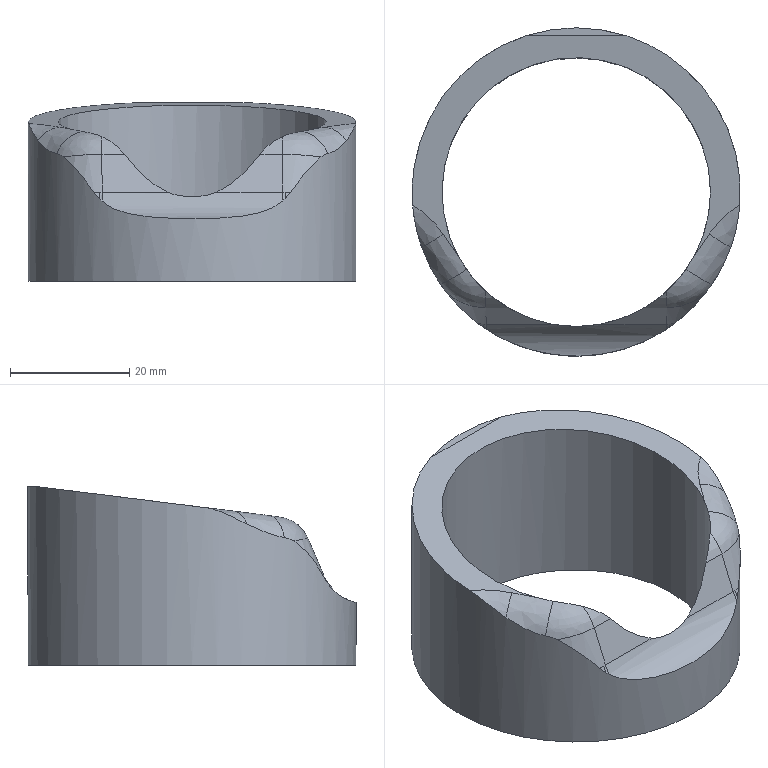Part | NX | features solid 2 | 1 solid | 22 faces | box 55 x 55 x 30 mm | volume 19165 mm3 | spline 10 | cylinder 7 | plane 5 | commonest cylinder face diameters 12 x2 20 x2 15 x1 45 x1 55 x1
STEP:
#1=CARTESIAN_POINT('',(-336.497,-154.34,29.));
#2=VERTEX_POINT('',#1);
#3=CARTESIAN_POINT('',(-353.503,-154.34,29.));
#4=VERTEX_POINT('',#3);
#5=CARTESIAN_POINT('',(-345.,-154.34,29.));
#6=DIRECTION('',(1.,0.,0.));
#7=VECTOR('',#6,1000.);
#8=LINE('',#5,#7);
#9=EDGE_CURVE('',#2,#4,#8,.F.);
#10=ORIENTED_EDGE('',*,*,#9,.F.);
#11=CARTESIAN_POINT('',(-345.,-180.493,29.));
#12=DIRECTION('',(0.,0.,1.));
#13=DIRECTION('',(1.,0.,0.));
#14=AXIS2_PLACEMENT_3D('',#11,#12,#13);
#15=CIRCLE('',#14,27.5);
#16=EDGE_CURVE('',#4,#2,#15,.F.);
#17=ORIENTED_EDGE('',*,*,#16,.F.);
#18=EDGE_LOOP('',(#10,#17));
#19=FACE_BOUND('',#18,.T.);
#20=CARTESIAN_POINT('',(-345.,-180.493,29.));
#21=DIRECTION('',(0.,0.,1.));
#22=DIRECTION('',(1.,0.,0.));
#23=AXIS2_PLACEMENT_3D('',#20,#21,#22);
#24=PLANE('',#23);
#25=ADVANCED_FACE('',(#19),#24,.T.);
#26=CARTESIAN_POINT('',(-322.5,-180.493,-1.));
#27=VERTEX_POINT('',#26);
#28=CARTESIAN_POINT('',(-345.,-180.493,-1.));
#29=DIRECTION('',(0.,0.,1.));
#30=DIRECTION('',(1.,0.,0.));
#31=AXIS2_PLACEMENT_3D('',#28,#29,#30);
#32=CIRCLE('',#31,22.5);
#33=EDGE_CURVE('',#27,#27,#32,.F.);
#34=ORIENTED_EDGE('',*,*,#33,.T.);
#35=EDGE_LOOP('',(#34));
#36=FACE_BOUND('',#35,.T.);
#37=CARTESIAN_POINT('',(-325.178,-191.138,24.41));
#38=VERTEX_POINT('',#37);
#39=CARTESIAN_POINT('',(-325.175,-191.134,24.41));
#40=VERTEX_POINT('',#39);
#41=CARTESIAN_POINT('',(-325.178,-191.138,24.41));
#42=CARTESIAN_POINT('',(-325.177,-191.137,24.41));
#43=CARTESIAN_POINT('',(-325.176,-191.135,24.41));
#44=CARTESIAN_POINT('',(-325.176,-191.134,24.41));
#45=B_SPLINE_CURVE_WITH_KNOTS('',3,(#41,#42,#43,#44),.UNSPECIFIED.,.F.,.F.,(4,4),(0.,1.),.UNSPECIFIED.);
#46=EDGE_CURVE('',#38,#40,#45,.T.);
#47=ORIENTED_EDGE('',*,*,#46,.T.);
#48=CARTESIAN_POINT('',(-364.825,-191.134,24.41));
#49=VERTEX_POINT('',#48);
#50=CARTESIAN_POINT('',(-345.,-180.493,25.738));
#51=DIRECTION('',(0.,-0.1238,0.9923));
#52=DIRECTION('',(0.,0.9923,0.1238));
#53=AXIS2_PLACEMENT_3D('',#50,#51,#52);
#54=ELLIPSE('',#53,22.674,22.5);
#55=EDGE_CURVE('',#40,#49,#54,.T.);
#56=ORIENTED_EDGE('',*,*,#55,.T.);
#57=CARTESIAN_POINT('',(-364.822,-191.138,24.41));
#58=VERTEX_POINT('',#57);
#59=CARTESIAN_POINT('',(-364.825,-191.134,24.41));
#60=CARTESIAN_POINT('',(-364.824,-191.135,24.41));
#61=CARTESIAN_POINT('',(-364.823,-191.136,24.41));
#62=CARTESIAN_POINT('',(-364.822,-191.138,24.41));
#63=B_SPLINE_CURVE_WITH_KNOTS('',3,(#59,#60,#61,#62),.UNSPECIFIED.,.F.,.F.,(4,4),(0.,1.),.UNSPECIFIED.);
#64=EDGE_CURVE('',#49,#58,#63,.T.);
#65=ORIENTED_EDGE('',*,*,#64,.T.);
#66=CARTESIAN_POINT('',(-363.388,-193.46,24.119));
#67=VERTEX_POINT('',#66);
#68=CARTESIAN_POINT('',(-364.822,-191.138,24.41));
#69=CARTESIAN_POINT('',(-364.391,-191.94,24.309));
#70=CARTESIAN_POINT('',(-363.913,-192.714,24.211));
#71=CARTESIAN_POINT('',(-363.388,-193.46,24.119));
#72=B_SPLINE_CURVE_WITH_KNOTS('',3,(#68,#69,#70,#71),.UNSPECIFIED.,.F.,.F.,(4,4),(0.000004606,0.00275),.UNSPECIFIED.);
#73=EDGE_CURVE('',#58,#67,#72,.T.);
#74=ORIENTED_EDGE('',*,*,#73,.T.);
#75=CARTESIAN_POINT('',(-360.131,-197.145,23.293));
#76=VERTEX_POINT('',#75);
#77=CARTESIAN_POINT('',(-363.388,-193.46,24.119));
#78=CARTESIAN_POINT('',(-362.429,-194.818,23.95));
#79=CARTESIAN_POINT('',(-361.302,-196.081,23.84));
#80=CARTESIAN_POINT('',(-360.131,-197.145,23.293));
#81=B_SPLINE_CURVE_WITH_KNOTS('',3,(#77,#78,#79,#80),.UNSPECIFIED.,.F.,.F.,(4,4),(0.,0.005011),.UNSPECIFIED.);
#82=EDGE_CURVE('',#67,#76,#81,.T.);
#83=ORIENTED_EDGE('',*,*,#82,.T.);
#84=CARTESIAN_POINT('',(-356.336,-199.928,20.3));
#85=VERTEX_POINT('',#84);
#86=CARTESIAN_POINT('',(-360.131,-197.145,23.293));
#87=CARTESIAN_POINT('',(-359.468,-197.747,22.984));
#88=CARTESIAN_POINT('',(-358.149,-198.805,22.193));
#89=CARTESIAN_POINT('',(-356.866,-199.619,21.027));
#90=CARTESIAN_POINT('',(-356.336,-199.928,20.3));
#91=B_SPLINE_CURVE_WITH_KNOTS('',3,(#86,#87,#88,#89,#90),.UNSPECIFIED.,.F.,.F.,(4,1,4),(0.,0.002803,0.005605),.UNSPECIFIED.);
#92=EDGE_CURVE('',#76,#85,#91,.T.);
#93=ORIENTED_EDGE('',*,*,#92,.T.);
#94=CARTESIAN_POINT('',(-349.112,-202.614,13.973));
#95=VERTEX_POINT('',#94);
#96=CARTESIAN_POINT('',(-345.,-180.493,66.089));
#97=DIRECTION('',(0.,0.9205,-0.3907));
#98=DIRECTION('',(0.,0.3907,0.9205));
#99=AXIS2_PLACEMENT_3D('',#96,#97,#98);
#100=ELLIPSE('',#99,57.586,22.5);
#101=EDGE_CURVE('',#95,#85,#100,.T.);
#102=ORIENTED_EDGE('',*,*,#101,.F.);
#103=CARTESIAN_POINT('',(-340.888,-202.614,13.973));
#104=VERTEX_POINT('',#103);
#105=CARTESIAN_POINT('',(-340.888,-202.614,13.973));
#106=CARTESIAN_POINT('',(-342.176,-202.853,13.409));
#107=CARTESIAN_POINT('',(-344.991,-203.132,13.001));
#108=CARTESIAN_POINT('',(-347.826,-202.853,13.41));
#109=CARTESIAN_POINT('',(-349.112,-202.614,13.973));
#110=B_SPLINE_CURVE_WITH_KNOTS('',3,(#105,#106,#107,#108,#109),.UNSPECIFIED.,.F.,.F.,(4,1,4),(0.,0.004206,0.008413),.UNSPECIFIED.);
#111=EDGE_CURVE('',#104,#95,#110,.T.);
#112=ORIENTED_EDGE('',*,*,#111,.F.);
#113=CARTESIAN_POINT('',(-333.664,-199.928,20.3));
#114=VERTEX_POINT('',#113);
#115=CARTESIAN_POINT('',(-345.,-180.493,66.089));
#116=DIRECTION('',(0.,0.9205,-0.3907));
#117=DIRECTION('',(0.,0.3907,0.9205));
#118=AXIS2_PLACEMENT_3D('',#115,#116,#117);
#119=ELLIPSE('',#118,57.586,22.5);
#120=EDGE_CURVE('',#114,#104,#119,.T.);
#121=ORIENTED_EDGE('',*,*,#120,.F.);
#122=CARTESIAN_POINT('',(-329.869,-197.145,23.293));
#123=VERTEX_POINT('',#122);
#124=CARTESIAN_POINT('',(-333.664,-199.928,20.3));
#125=CARTESIAN_POINT('',(-332.603,-199.309,21.757));
#126=CARTESIAN_POINT('',(-331.194,-198.348,22.676));
#127=CARTESIAN_POINT('',(-329.869,-197.145,23.293));
#128=B_SPLINE_CURVE_WITH_KNOTS('',3,(#124,#125,#126,#127),.UNSPECIFIED.,.F.,.F.,(4,4),(0.,0.00561),.UNSPECIFIED.);
#129=EDGE_CURVE('',#114,#123,#128,.T.);
#130=ORIENTED_EDGE('',*,*,#129,.T.);
#131=CARTESIAN_POINT('',(-326.612,-193.46,24.119));
#132=VERTEX_POINT('',#131);
#133=CARTESIAN_POINT('',(-329.869,-197.145,23.293));
#134=CARTESIAN_POINT('',(-328.699,-196.082,23.839));
#135=CARTESIAN_POINT('',(-327.57,-194.818,23.95));
#136=CARTESIAN_POINT('',(-326.612,-193.46,24.119));
#137=B_SPLINE_CURVE_WITH_KNOTS('',3,(#133,#134,#135,#136),.UNSPECIFIED.,.F.,.F.,(4,4),(0.,0.005002),.UNSPECIFIED.);
#138=EDGE_CURVE('',#123,#132,#137,.T.);
#139=ORIENTED_EDGE('',*,*,#138,.T.);
#140=CARTESIAN_POINT('',(-326.612,-193.46,24.119));
#141=CARTESIAN_POINT('',(-326.087,-192.715,24.211));
#142=CARTESIAN_POINT('',(-325.609,-191.941,24.309));
#143=CARTESIAN_POINT('',(-325.178,-191.138,24.41));
#144=B_SPLINE_CURVE_WITH_KNOTS('',3,(#140,#141,#142,#143),.UNSPECIFIED.,.F.,.F.,(4,4),(0.,0.002745),.UNSPECIFIED.);
#145=EDGE_CURVE('',#132,#38,#144,.T.);
#146=ORIENTED_EDGE('',*,*,#145,.T.);
#147=EDGE_LOOP('',(#47,#56,#65,#74,#83,#93,#102,#112,#121,#130,#139,#146));
#148=FACE_BOUND('',#147,.T.);
#149=CARTESIAN_POINT('',(-345.,-180.493,-1.));
#150=DIRECTION('',(0.,0.,1.));
#151=DIRECTION('',(1.,0.,0.));
#152=AXIS2_PLACEMENT_3D('',#149,#150,#151);
#153=CYLINDRICAL_SURFACE('',#152,22.5);
#154=ADVANCED_FACE('',(#36,#148),#153,.F.);
#155=CARTESIAN_POINT('',(-372.5,-180.493,-1.));
#156=VERTEX_POINT('',#155);
#157=CARTESIAN_POINT('',(-345.,-180.493,-1.));
#158=DIRECTION('',(0.,0.,-1.));
#159=DIRECTION('',(-1.,0.,0.));
#160=AXIS2_PLACEMENT_3D('',#157,#158,#159);
#161=CIRCLE('',#160,27.5);
#162=EDGE_CURVE('',#156,#156,#161,.T.);
#163=ORIENTED_EDGE('',*,*,#162,.F.);
#164=EDGE_LOOP('',(#163));
#165=FACE_BOUND('',#164,.T.);
#166=CARTESIAN_POINT('',(-372.414,-182.672,25.466));
#167=VERTEX_POINT('',#166);
#168=CARTESIAN_POINT('',(-345.,-180.493,25.738));
#169=DIRECTION('',(0.,-0.1238,0.9923));
#170=DIRECTION('',(0.,0.9923,0.1238));
#171=AXIS2_PLACEMENT_3D('',#168,#169,#170);
#172=ELLIPSE('',#171,27.713,27.5);
#173=EDGE_CURVE('',#4,#167,#172,.T.);
#174=ORIENTED_EDGE('',*,*,#173,.F.);
#175=ORIENTED_EDGE('',*,*,#16,.T.);
#176=CARTESIAN_POINT('',(-317.585,-182.649,25.469));
#177=VERTEX_POINT('',#176);
#178=CARTESIAN_POINT('',(-345.,-180.493,25.738));
#179=DIRECTION('',(0.,-0.1238,0.9923));
#180=DIRECTION('',(0.,0.9923,0.1238));
#181=AXIS2_PLACEMENT_3D('',#178,#179,#180);
#182=ELLIPSE('',#181,27.713,27.5);
#183=EDGE_CURVE('',#177,#2,#182,.T.);
#184=ORIENTED_EDGE('',*,*,#183,.F.);
#185=CARTESIAN_POINT('',(-319.108,-189.759,22.675));
#186=VERTEX_POINT('',#185);
#187=CARTESIAN_POINT('',(-319.108,-189.759,22.675));
#188=CARTESIAN_POINT('',(-318.29,-187.473,23.676));
#189=CARTESIAN_POINT('',(-317.79,-185.264,25.142));
#190=CARTESIAN_POINT('',(-317.585,-182.649,25.469));
#191=B_SPLINE_CURVE_WITH_KNOTS('',3,(#187,#188,#189,#190),.UNSPECIFIED.,.F.,.F.,(4,4),(0.,0.007856),.UNSPECIFIED.);
#192=EDGE_CURVE('',#186,#177,#191,.T.);
#193=ORIENTED_EDGE('',*,*,#192,.F.);
#194=CARTESIAN_POINT('',(-322.27,-195.971,20.446));
#195=VERTEX_POINT('',#194);
#196=CARTESIAN_POINT('',(-322.27,-195.971,20.446));
#197=CARTESIAN_POINT('',(-320.893,-193.95,20.709));
#198=CARTESIAN_POINT('',(-319.874,-191.897,21.738));
#199=CARTESIAN_POINT('',(-319.108,-189.759,22.675));
#200=B_SPLINE_CURVE_WITH_KNOTS('',3,(#196,#197,#198,#199),.UNSPECIFIED.,.F.,.F.,(4,4),(0.,0.007347),.UNSPECIFIED.);
#201=EDGE_CURVE('',#195,#186,#200,.T.);
#202=ORIENTED_EDGE('',*,*,#201,.F.);
#203=CARTESIAN_POINT('',(-323.445,-197.569,19.879));
#204=VERTEX_POINT('',#203);
#205=CARTESIAN_POINT('',(-323.446,-197.571,19.878));
#206=CARTESIAN_POINT('',(-323.058,-197.082,20.202));
#207=CARTESIAN_POINT('',(-322.661,-196.546,20.37));
#208=CARTESIAN_POINT('',(-322.27,-195.971,20.446));
#209=B_SPLINE_CURVE_WITH_KNOTS('',3,(#205,#206,#207,#208),.UNSPECIFIED.,.F.,.F.,(4,4),(0.,0.002064),.UNSPECIFIED.);
#210=EDGE_CURVE('',#204,#195,#209,.T.);
#211=ORIENTED_EDGE('',*,*,#210,.F.);
#212=CARTESIAN_POINT('',(-328.545,-202.527,13.948));
#213=VERTEX_POINT('',#212);
#214=CARTESIAN_POINT('',(-328.546,-202.527,13.947));
#215=CARTESIAN_POINT('',(-327.725,-201.914,15.109));
#216=CARTESIAN_POINT('',(-326.053,-200.526,17.284));
#217=CARTESIAN_POINT('',(-324.311,-198.663,19.156));
#218=CARTESIAN_POINT('',(-323.443,-197.568,19.88));
#219=B_SPLINE_CURVE_WITH_KNOTS('',3,(#214,#215,#216,#217,#218),.UNSPECIFIED.,.F.,.F.,(4,1,4),(0.002663,0.007292,0.01192),.UNSPECIFIED.);
#220=EDGE_CURVE('',#213,#204,#219,.T.);
#221=ORIENTED_EDGE('',*,*,#220,.F.);
#222=CARTESIAN_POINT('',(-329.415,-203.15,12.923));
#223=VERTEX_POINT('',#222);
#224=CARTESIAN_POINT('',(-328.545,-202.526,13.948));
#225=CARTESIAN_POINT('',(-328.808,-202.723,13.576));
#226=CARTESIAN_POINT('',(-329.103,-202.935,13.242));
#227=CARTESIAN_POINT('',(-329.415,-203.15,12.923));
#228=B_SPLINE_CURVE_WITH_KNOTS('',3,(#224,#225,#226,#227),.UNSPECIFIED.,.F.,.F.,(4,4),(0.,0.001482),.UNSPECIFIED.);
#229=EDGE_CURVE('',#213,#223,#228,.T.);
#230=ORIENTED_EDGE('',*,*,#229,.T.);
#231=CARTESIAN_POINT('',(-329.884,-203.466,12.473));
#232=VERTEX_POINT('',#231);
#233=CARTESIAN_POINT('',(-329.415,-203.15,12.923));
#234=CARTESIAN_POINT('',(-329.567,-203.254,12.768));
#235=CARTESIAN_POINT('',(-329.723,-203.36,12.618));
#236=CARTESIAN_POINT('',(-329.884,-203.466,12.473));
#237=B_SPLINE_CURVE_WITH_KNOTS('',3,(#233,#234,#235,#236),.UNSPECIFIED.,.F.,.F.,(4,4),(0.,0.0007229),.UNSPECIFIED.);
#238=EDGE_CURVE('',#223,#232,#237,.T.);
#239=ORIENTED_EDGE('',*,*,#238,.T.);
#240=CARTESIAN_POINT('',(-360.116,-203.466,12.473));
#241=VERTEX_POINT('',#240);
#242=CARTESIAN_POINT('',(-329.884,-203.466,12.473));
#243=CARTESIAN_POINT('',(-330.82,-204.081,11.633));
#244=CARTESIAN_POINT('',(-333.044,-205.367,10.549));
#245=CARTESIAN_POINT('',(-338.129,-207.366,9.625));
#246=CARTESIAN_POINT('',(-343.602,-208.202,9.529));
#247=CARTESIAN_POINT('',(-349.134,-207.783,9.598));
#248=CARTESIAN_POINT('',(-353.106,-206.876,9.848));
#249=CARTESIAN_POINT('',(-356.94,-205.377,10.543));
#250=CARTESIAN_POINT('',(-359.182,-204.08,11.634));
#251=CARTESIAN_POINT('',(-360.116,-203.466,12.473));
#252=B_SPLINE_CURVE_WITH_KNOTS('',3,(#242,#243,#244,#245,#246,#247,#248,#249,#250,#251),.UNSPECIFIED.,.F.,.F.,(4,1,1,1,1,1,1,4),(0.,0.00412,0.00824,0.01648,0.0206,0.02472,0.02884,0.03296),.UNSPECIFIED.);
#253=EDGE_CURVE('',#232,#241,#252,.T.);
#254=ORIENTED_EDGE('',*,*,#253,.T.);
#255=CARTESIAN_POINT('',(-360.585,-203.15,12.923));
#256=VERTEX_POINT('',#255);
#257=CARTESIAN_POINT('',(-360.116,-203.466,12.473));
#258=CARTESIAN_POINT('',(-360.277,-203.36,12.618));
#259=CARTESIAN_POINT('',(-360.433,-203.254,12.768));
#260=CARTESIAN_POINT('',(-360.585,-203.15,12.923));
#261=B_SPLINE_CURVE_WITH_KNOTS('',3,(#257,#258,#259,#260),.UNSPECIFIED.,.F.,.F.,(4,4),(0.,0.0007229),.UNSPECIFIED.);
#262=EDGE_CURVE('',#241,#256,#261,.T.);
#263=ORIENTED_EDGE('',*,*,#262,.T.);
#264=CARTESIAN_POINT('',(-361.455,-202.526,13.948));
#265=VERTEX_POINT('',#264);
#266=CARTESIAN_POINT('',(-360.585,-203.15,12.923));
#267=CARTESIAN_POINT('',(-360.897,-202.935,13.242));
#268=CARTESIAN_POINT('',(-361.192,-202.723,13.576));
#269=CARTESIAN_POINT('',(-361.455,-202.526,13.948));
#270=B_SPLINE_CURVE_WITH_KNOTS('',3,(#266,#267,#268,#269),.UNSPECIFIED.,.F.,.F.,(4,4),(0.,0.001482),.UNSPECIFIED.);
#271=EDGE_CURVE('',#256,#265,#270,.T.);
#272=ORIENTED_EDGE('',*,*,#271,.T.);
#273=CARTESIAN_POINT('',(-366.556,-197.569,19.879));
#274=VERTEX_POINT('',#273);
#275=CARTESIAN_POINT('',(-366.557,-197.568,19.88));
#276=CARTESIAN_POINT('',(-364.834,-199.742,18.443));
#277=CARTESIAN_POINT('',(-363.1,-201.298,16.275));
#278=CARTESIAN_POINT('',(-361.454,-202.527,13.948));
#279=B_SPLINE_CURVE_WITH_KNOTS('',3,(#275,#276,#277,#278),.UNSPECIFIED.,.F.,.F.,(4,4),(0.0005928,0.009901),.UNSPECIFIED.);
#280=EDGE_CURVE('',#274,#265,#279,.T.);
#281=ORIENTED_EDGE('',*,*,#280,.F.);
#282=CARTESIAN_POINT('',(-367.73,-195.971,20.445));
#283=VERTEX_POINT('',#282);
#284=CARTESIAN_POINT('',(-367.73,-195.971,20.445));
#285=CARTESIAN_POINT('',(-367.339,-196.545,20.37));
#286=CARTESIAN_POINT('',(-366.942,-197.082,20.202));
#287=CARTESIAN_POINT('',(-366.554,-197.571,19.878));
#288=B_SPLINE_CURVE_WITH_KNOTS('',3,(#284,#285,#286,#287),.UNSPECIFIED.,.F.,.F.,(4,4),(0.,0.002064),.UNSPECIFIED.);
#289=EDGE_CURVE('',#283,#274,#288,.T.);
#290=ORIENTED_EDGE('',*,*,#289,.F.);
#291=CARTESIAN_POINT('',(-370.892,-189.759,22.675));
#292=VERTEX_POINT('',#291);
#293=CARTESIAN_POINT('',(-370.892,-189.759,22.675));
#294=CARTESIAN_POINT('',(-370.127,-191.897,21.738));
#295=CARTESIAN_POINT('',(-369.107,-193.95,20.709));
#296=CARTESIAN_POINT('',(-367.73,-195.971,20.445));
#297=B_SPLINE_CURVE_WITH_KNOTS('',3,(#293,#294,#295,#296),.UNSPECIFIED.,.F.,.F.,(4,4),(0.,0.00736),.UNSPECIFIED.);
#298=EDGE_CURVE('',#292,#283,#297,.T.);
#299=ORIENTED_EDGE('',*,*,#298,.F.);
#300=CARTESIAN_POINT('',(-372.413,-182.672,25.466));
#301=CARTESIAN_POINT('',(-372.31,-183.974,25.303));
#302=CARTESIAN_POINT('',(-371.932,-186.41,24.445));
#303=CARTESIAN_POINT('',(-371.299,-188.62,23.174));
#304=CARTESIAN_POINT('',(-370.892,-189.759,22.675));
#305=B_SPLINE_CURVE_WITH_KNOTS('',3,(#300,#301,#302,#303,#304),.UNSPECIFIED.,.F.,.F.,(4,1,4),(0.,0.003887,0.007775),.UNSPECIFIED.);
#306=EDGE_CURVE('',#167,#292,#305,.T.);
#307=ORIENTED_EDGE('',*,*,#306,.F.);
#308=EDGE_LOOP('',(#174,#175,#184,#193,#202,#211,#221,#230,#239,#254,#263,#272,#281,#290,#299,#307));
#309=FACE_BOUND('',#308,.T.);
#310=CARTESIAN_POINT('',(-345.,-180.493,-1.));
#311=DIRECTION('',(0.,0.,1.));
#312=DIRECTION('',(1.,0.,0.));
#313=AXIS2_PLACEMENT_3D('',#310,#311,#312);
#314=CYLINDRICAL_SURFACE('',#313,27.5);
#315=ADVANCED_FACE('',(#165,#309),#314,.T.);
#316=ORIENTED_EDGE('',*,*,#33,.F.);
#317=EDGE_LOOP('',(#316));
#318=FACE_BOUND('',#317,.T.);
#319=ORIENTED_EDGE('',*,*,#162,.T.);
#320=EDGE_LOOP('',(#319));
#321=FACE_BOUND('',#320,.T.);
#322=CARTESIAN_POINT('',(-345.,-180.493,-1.));
#323=DIRECTION('',(0.,0.,1.));
#324=DIRECTION('',(1.,0.,0.));
#325=AXIS2_PLACEMENT_3D('',#322,#323,#324);
#326=PLANE('',#325);
#327=ADVANCED_FACE('',(#318,#321),#326,.F.);
#328=ORIENTED_EDGE('',*,*,#92,.F.);
#329=CARTESIAN_POINT('',(-360.131,-199.928,20.3));
#330=VERTEX_POINT('',#329);
#331=CARTESIAN_POINT('',(-360.131,-197.145,23.293));
#332=CARTESIAN_POINT('',(-360.131,-198.382,22.658));
#333=CARTESIAN_POINT('',(-360.131,-199.385,21.58));
#334=CARTESIAN_POINT('',(-360.131,-199.928,20.3));
#335=B_SPLINE_CURVE_WITH_KNOTS('',3,(#331,#332,#333,#334),.UNSPECIFIED.,.F.,.F.,(4,4),(0.335,1.),.UNSPECIFIED.);
#336=EDGE_CURVE('',#76,#330,#335,.T.);
#337=ORIENTED_EDGE('',*,*,#336,.T.);
#338=CARTESIAN_POINT('',(-360.131,-199.928,20.3));
#339=CARTESIAN_POINT('',(-358.866,-199.928,20.3));
#340=CARTESIAN_POINT('',(-357.601,-199.928,20.3));
#341=CARTESIAN_POINT('',(-356.336,-199.928,20.3));
#342=B_SPLINE_CURVE_WITH_KNOTS('',3,(#338,#339,#340,#341),.UNSPECIFIED.,.F.,.F.,(4,4),(0.,0.1254),.UNSPECIFIED.);
#343=EDGE_CURVE('',#330,#85,#342,.T.);
#344=ORIENTED_EDGE('',*,*,#343,.T.);
#345=EDGE_LOOP('',(#328,#337,#344));
#346=FACE_BOUND('',#345,.T.);
#347=CARTESIAN_POINT('',(-354.079,-194.405,17.955));
#348=DIRECTION('',(-1.,0.,0.));
#349=DIRECTION('',(0.,0.,-1.));
#350=AXIS2_PLACEMENT_3D('',#347,#348,#349);
#351=CYLINDRICAL_SURFACE('',#350,6.);
#352=ADVANCED_FACE('',(#346),#351,.T.);
#353=CARTESIAN_POINT('',(-329.869,-199.928,20.3));
#354=VERTEX_POINT('',#353);
#355=CARTESIAN_POINT('',(-333.664,-199.928,20.3));
#356=CARTESIAN_POINT('',(-332.399,-199.928,20.3));
#357=CARTESIAN_POINT('',(-331.134,-199.928,20.3));
#358=CARTESIAN_POINT('',(-329.869,-199.928,20.3));
#359=B_SPLINE_CURVE_WITH_KNOTS('',3,(#355,#356,#357,#358),.UNSPECIFIED.,.F.,.F.,(4,4),(0.8746,1.),.UNSPECIFIED.);
#360=EDGE_CURVE('',#114,#354,#359,.T.);
#361=ORIENTED_EDGE('',*,*,#360,.F.);
#362=ORIENTED_EDGE('',*,*,#120,.T.);
#363=CARTESIAN_POINT('',(-329.884,-202.612,13.976));
#364=VERTEX_POINT('',#363);
#365=CARTESIAN_POINT('',(-329.884,-202.614,13.973));
#366=CARTESIAN_POINT('',(-333.552,-202.614,13.973));
#367=CARTESIAN_POINT('',(-337.22,-202.614,13.973));
#368=CARTESIAN_POINT('',(-340.888,-202.614,13.973));
#369=B_SPLINE_CURVE_WITH_KNOTS('',3,(#365,#366,#367,#368),.UNSPECIFIED.,.F.,.F.,(4,4),(0.,0.364),.UNSPECIFIED.);
#370=EDGE_CURVE('',#364,#104,#369,.T.);
#371=ORIENTED_EDGE('',*,*,#370,.F.);
#372=CARTESIAN_POINT('',(-329.869,-199.928,20.3));
#373=CARTESIAN_POINT('',(-329.874,-200.823,18.193));
#374=CARTESIAN_POINT('',(-329.879,-201.717,16.086));
#375=CARTESIAN_POINT('',(-329.884,-202.611,13.978));
#376=B_SPLINE_CURVE_WITH_KNOTS('',3,(#372,#373,#374,#375),.UNSPECIFIED.,.F.,.F.,(4,4),(0.,0.9992),.UNSPECIFIED.);
#377=EDGE_CURVE('',#354,#364,#376,.T.);
#378=ORIENTED_EDGE('',*,*,#377,.F.);
#379=EDGE_LOOP('',(#361,#362,#371,#378));
#380=FACE_BOUND('',#379,.T.);
#381=CARTESIAN_POINT('',(-329.688,-199.928,20.3));
#382=DIRECTION('',(0.,0.9205,-0.3907));
#383=DIRECTION('',(0.,-0.3907,-0.9205));
#384=AXIS2_PLACEMENT_3D('',#381,#382,#383);
#385=PLANE('',#384);
#386=ADVANCED_FACE('',(#380),#385,.F.);
#387=ORIENTED_EDGE('',*,*,#55,.F.);
#388=CARTESIAN_POINT('',(-322.725,-187.554,24.857));
#389=VERTEX_POINT('',#388);
#390=CARTESIAN_POINT('',(-325.175,-191.134,24.41));
#391=CARTESIAN_POINT('',(-324.359,-189.941,24.559));
#392=CARTESIAN_POINT('',(-323.542,-188.748,24.708));
#393=CARTESIAN_POINT('',(-322.725,-187.555,24.857));
#394=B_SPLINE_CURVE_WITH_KNOTS('',3,(#390,#391,#392,#393),.UNSPECIFIED.,.F.,.F.,(4,4),(0.3864,1.),.UNSPECIFIED.);
#395=EDGE_CURVE('',#40,#389,#394,.T.);
#396=ORIENTED_EDGE('',*,*,#395,.T.);
#397=CARTESIAN_POINT('',(-322.725,-187.554,24.857));
#398=CARTESIAN_POINT('',(-322.612,-187.391,24.877));
#399=CARTESIAN_POINT('',(-322.48,-187.202,24.901));
#400=CARTESIAN_POINT('',(-322.111,-186.702,24.963));
#401=CARTESIAN_POINT('',(-321.652,-186.128,25.035));
#402=CARTESIAN_POINT('',(-321.052,-185.449,25.119));
#403=CARTESIAN_POINT('',(-320.222,-184.607,25.224));
#404=CARTESIAN_POINT('',(-319.082,-183.625,25.347));
#405=CARTESIAN_POINT('',(-318.097,-182.957,25.43));
#406=CARTESIAN_POINT('',(-317.585,-182.649,25.469));
#407=B_SPLINE_CURVE_WITH_KNOTS('',3,(#397,#398,#399,#400,#401,#402,#403,#404,#405,#406),.UNSPECIFIED.,.F.,.F.,(4,1,1,1,1,1,1,4),(0.,0.02988,0.05976,0.1195,0.1793,0.239,0.3586,0.4781),.UNSPECIFIED.);
#408=EDGE_CURVE('',#389,#177,#407,.T.);
#409=ORIENTED_EDGE('',*,*,#408,.T.);
#410=ORIENTED_EDGE('',*,*,#183,.T.);
#411=ORIENTED_EDGE('',*,*,#9,.T.);
#412=ORIENTED_EDGE('',*,*,#173,.T.);
#413=CARTESIAN_POINT('',(-367.275,-187.554,24.857));
#414=VERTEX_POINT('',#413);
#415=CARTESIAN_POINT('',(-372.413,-182.671,25.466));
#416=CARTESIAN_POINT('',(-371.908,-182.975,25.428));
#417=CARTESIAN_POINT('',(-370.918,-183.651,25.344));
#418=CARTESIAN_POINT('',(-369.781,-184.625,25.222));
#419=CARTESIAN_POINT('',(-368.944,-185.466,25.117));
#420=CARTESIAN_POINT('',(-368.346,-186.137,25.033));
#421=CARTESIAN_POINT('',(-367.888,-186.704,24.963));
#422=CARTESIAN_POINT('',(-367.528,-187.196,24.901));
#423=CARTESIAN_POINT('',(-367.389,-187.392,24.877));
#424=CARTESIAN_POINT('',(-367.275,-187.554,24.857));
#425=B_SPLINE_CURVE_WITH_KNOTS('',3,(#415,#416,#417,#418,#419,#420,#421,#422,#423,#424),.UNSPECIFIED.,.F.,.F.,(4,1,1,1,1,1,1,4),(0.2869,0.4652,0.6435,0.7326,0.8217,0.9109,0.9554,1.),.UNSPECIFIED.);
#426=EDGE_CURVE('',#167,#414,#425,.T.);
#427=ORIENTED_EDGE('',*,*,#426,.T.);
#428=CARTESIAN_POINT('',(-367.275,-187.555,24.857));
#429=CARTESIAN_POINT('',(-366.458,-188.748,24.708));
#430=CARTESIAN_POINT('',(-365.642,-189.941,24.559));
#431=CARTESIAN_POINT('',(-364.825,-191.134,24.41));
#432=B_SPLINE_CURVE_WITH_KNOTS('',3,(#428,#429,#430,#431),.UNSPECIFIED.,.F.,.F.,(4,4),(0.,0.6135),.UNSPECIFIED.);
#433=EDGE_CURVE('',#414,#49,#432,.T.);
#434=ORIENTED_EDGE('',*,*,#433,.T.);
#435=EDGE_LOOP('',(#387,#396,#409,#410,#411,#412,#427,#434));
#436=FACE_BOUND('',#435,.T.);
#437=CARTESIAN_POINT('',(-300.,-111.421,34.354));
#438=DIRECTION('',(0.,-0.1238,0.9923));
#439=DIRECTION('',(0.,0.9923,0.1238));
#440=AXIS2_PLACEMENT_3D('',#437,#438,#439);
#441=PLANE('',#440);
#442=ADVANCED_FACE('',(#436),#441,.T.);
#443=CARTESIAN_POINT('',(-322.725,-187.555,24.857));
#444=CARTESIAN_POINT('',(-321.471,-188.401,24.751));
#445=CARTESIAN_POINT('',(-320.05,-189.274,23.957));
#446=CARTESIAN_POINT('',(-319.108,-189.759,22.675));
#447=B_SPLINE_CURVE_WITH_KNOTS('',3,(#443,#444,#445,#446),.UNSPECIFIED.,.F.,.F.,(4,4),(0.,0.6439),.UNSPECIFIED.);
#448=EDGE_CURVE('',#389,#186,#447,.T.);
#449=ORIENTED_EDGE('',*,*,#448,.T.);
#450=ORIENTED_EDGE('',*,*,#192,.T.);
#451=ORIENTED_EDGE('',*,*,#408,.F.);
#452=EDGE_LOOP('',(#449,#450,#451));
#453=FACE_BOUND('',#452,.T.);
#454=CARTESIAN_POINT('',(-319.092,-189.768,22.652));
#455=CARTESIAN_POINT('',(-320.564,-189.012,24.675));
#456=CARTESIAN_POINT('',(-322.725,-187.555,24.857));
#457=CARTESIAN_POINT('',(-318.855,-189.357,22.746));
#458=CARTESIAN_POINT('',(-320.288,-188.548,24.733));
#459=CARTESIAN_POINT('',(-322.37,-187.036,24.921));
#460=CARTESIAN_POINT('',(-318.598,-188.962,22.837));
#461=CARTESIAN_POINT('',(-319.99,-188.103,24.788));
#462=CARTESIAN_POINT('',(-321.991,-186.539,24.983));
#463=CARTESIAN_POINT('',(-318.046,-188.207,23.009));
#464=CARTESIAN_POINT('',(-319.347,-187.251,24.895));
#465=CARTESIAN_POINT('',(-321.183,-185.592,25.101));
#466=CARTESIAN_POINT('',(-317.75,-187.847,23.091));
#467=CARTESIAN_POINT('',(-319.002,-186.844,24.945));
#468=CARTESIAN_POINT('',(-320.755,-185.142,25.158));
#469=CARTESIAN_POINT('',(-317.119,-187.163,23.245));
#470=CARTESIAN_POINT('',(-318.267,-186.072,25.041));
#471=CARTESIAN_POINT('',(-319.849,-184.288,25.264));
#472=CARTESIAN_POINT('',(-316.783,-186.839,23.318));
#473=CARTESIAN_POINT('',(-317.875,-185.707,25.087));
#474=CARTESIAN_POINT('',(-319.37,-183.885,25.314));
#475=CARTESIAN_POINT('',(-316.123,-186.281,23.444));
#476=CARTESIAN_POINT('',(-317.108,-185.077,25.166));
#477=CARTESIAN_POINT('',(-318.437,-183.19,25.401));
#478=CARTESIAN_POINT('',(-315.812,-186.044,23.497));
#479=CARTESIAN_POINT('',(-316.745,-184.81,25.199));
#480=CARTESIAN_POINT('',(-317.998,-182.897,25.438));
#481=CARTESIAN_POINT('',(-315.49,-185.827,23.545));
#482=CARTESIAN_POINT('',(-316.37,-184.565,25.23));
#483=CARTESIAN_POINT('',(-317.548,-182.627,25.471));
#484=(BOUNDED_SURFACE()B_SPLINE_SURFACE(3,2,((#454,#455,#456),(#457,#458,#459),(#460,#461,#462),(#463,#464,#465),(#466,#467,#468),(#469,#470,#471),(#472,#473,#474),(#475,#476,#477),(#478,#479,#480),(#481,#482,#483)),.UNSPECIFIED.,.F.,.F.,.F.)B_SPLINE_SURFACE_WITH_KNOTS((4,2,2,2,4),(3,3),(0.,0.125,0.25,0.375,0.4803),(0.3522,1.),.UNSPECIFIED.)GEOMETRIC_REPRESENTATION_ITEM()RATIONAL_B_SPLINE_SURFACE(((0.9125,0.8758,1.),(0.9145,0.8786,1.),(0.9164,0.8813,1.),(0.9199,0.8863,1.),(0.9216,0.8887,1.),(0.9248,0.8932,1.),(0.9263,0.8953,1.),(0.9288,0.8989,1.),(0.9299,0.9005,1.),(0.9309,0.9018,1.)))REPRESENTATION_ITEM('')SURFACE());
#485=ADVANCED_FACE('',(#453),#484,.T.);
#486=ORIENTED_EDGE('',*,*,#145,.F.);
#487=CARTESIAN_POINT('',(-326.612,-193.46,24.119));
#488=CARTESIAN_POINT('',(-325.77,-194.024,24.026));
#489=CARTESIAN_POINT('',(-323.94,-195.182,23.267));
#490=CARTESIAN_POINT('',(-322.658,-195.827,21.416));
#491=CARTESIAN_POINT('',(-322.27,-195.971,20.446));
#492=B_SPLINE_CURVE_WITH_KNOTS('',3,(#487,#488,#489,#490,#491),.UNSPECIFIED.,.F.,.F.,(4,1,4),(0.01803,0.4478,0.8775),.UNSPECIFIED.);
#493=EDGE_CURVE('',#132,#195,#492,.T.);
#494=ORIENTED_EDGE('',*,*,#493,.T.);
#495=ORIENTED_EDGE('',*,*,#201,.T.);
#496=ORIENTED_EDGE('',*,*,#448,.F.);
#497=ORIENTED_EDGE('',*,*,#395,.F.);
#498=ORIENTED_EDGE('',*,*,#46,.F.);
#499=EDGE_LOOP('',(#486,#494,#495,#496,#497,#498));
#500=FACE_BOUND('',#499,.T.);
#501=CARTESIAN_POINT('',(-322.256,-195.977,20.41));
#502=CARTESIAN_POINT('',(-323.616,-195.478,23.868));
#503=CARTESIAN_POINT('',(-326.718,-193.389,24.129));
#504=CARTESIAN_POINT('',(-320.925,-194.033,20.65));
#505=CARTESIAN_POINT('',(-322.284,-193.535,24.111));
#506=CARTESIAN_POINT('',(-325.388,-191.444,24.371));
#507=CARTESIAN_POINT('',(-319.594,-192.09,20.89));
#508=CARTESIAN_POINT('',(-320.952,-191.592,24.353));
#509=CARTESIAN_POINT('',(-324.057,-189.499,24.614));
#510=CARTESIAN_POINT('',(-318.262,-190.146,21.13));
#511=CARTESIAN_POINT('',(-319.62,-189.649,24.595));
#512=CARTESIAN_POINT('',(-322.725,-187.555,24.857));
#513=(BOUNDED_SURFACE()B_SPLINE_SURFACE(3,2,((#501,#502,#503),(#504,#505,#506),(#507,#508,#509),(#510,#511,#512)),.UNSPECIFIED.,.F.,.F.,.F.)B_SPLINE_SURFACE_WITH_KNOTS((4,4),(3,3),(0.,1.),(0.1172,1.),.PIECEWISE_BEZIER_KNOTS.)GEOMETRIC_REPRESENTATION_ITEM()RATIONAL_B_SPLINE_SURFACE(((0.9604,0.8311,1.),(0.9604,0.8309,1.),(0.9603,0.8308,1.),(0.9603,0.8307,1.)))REPRESENTATION_ITEM('')SURFACE());
#514=ADVANCED_FACE('',(#500),#513,.T.);
#515=ORIENTED_EDGE('',*,*,#138,.F.);
#516=CARTESIAN_POINT('',(-329.869,-199.928,20.3));
#517=CARTESIAN_POINT('',(-329.869,-199.385,21.58));
#518=CARTESIAN_POINT('',(-329.869,-198.382,22.658));
#519=CARTESIAN_POINT('',(-329.869,-197.145,23.293));
#520=B_SPLINE_CURVE_WITH_KNOTS('',3,(#516,#517,#518,#519),.UNSPECIFIED.,.F.,.F.,(4,4),(0.,0.665),.UNSPECIFIED.);
#521=EDGE_CURVE('',#123,#354,#520,.F.);
#522=ORIENTED_EDGE('',*,*,#521,.T.);
#523=CARTESIAN_POINT('',(-323.445,-197.569,19.88));
#524=CARTESIAN_POINT('',(-323.883,-197.939,19.947));
#525=CARTESIAN_POINT('',(-324.849,-198.623,20.07));
#526=CARTESIAN_POINT('',(-326.172,-199.244,20.18));
#527=CARTESIAN_POINT('',(-327.278,-199.596,20.242));
#528=CARTESIAN_POINT('',(-328.121,-199.786,20.275));
#529=CARTESIAN_POINT('',(-328.861,-199.885,20.292));
#530=CARTESIAN_POINT('',(-329.437,-199.921,20.298));
#531=CARTESIAN_POINT('',(-329.674,-199.928,20.3));
#532=CARTESIAN_POINT('',(-329.869,-199.928,20.3));
#533=B_SPLINE_CURVE_WITH_KNOTS('',3,(#523,#524,#525,#526,#527,#528,#529,#530,#531,#532),.UNSPECIFIED.,.F.,.F.,(4,1,1,1,1,1,1,4),(0.2319,0.424,0.616,0.712,0.808,0.904,0.952,1.),.UNSPECIFIED.);
#534=EDGE_CURVE('',#354,#204,#533,.F.);
#535=ORIENTED_EDGE('',*,*,#534,.T.);
#536=ORIENTED_EDGE('',*,*,#210,.T.);
#537=ORIENTED_EDGE('',*,*,#493,.F.);
#538=EDGE_LOOP('',(#515,#522,#535,#536,#537));
#539=FACE_BOUND('',#538,.T.);
#540=CARTESIAN_POINT('',(-329.869,-199.928,20.3));
#541=CARTESIAN_POINT('',(-329.869,-198.596,23.439));
#542=CARTESIAN_POINT('',(-329.869,-195.217,23.9));
#543=CARTESIAN_POINT('',(-329.077,-199.929,20.299));
#544=CARTESIAN_POINT('',(-329.234,-198.596,23.439));
#545=CARTESIAN_POINT('',(-329.546,-195.217,23.9));
#546=CARTESIAN_POINT('',(-328.305,-199.835,20.281));
#547=CARTESIAN_POINT('',(-328.614,-198.533,23.446));
#548=CARTESIAN_POINT('',(-329.231,-195.174,23.906));
#549=CARTESIAN_POINT('',(-327.361,-199.608,20.24));
#550=CARTESIAN_POINT('',(-327.846,-198.377,23.465));
#551=CARTESIAN_POINT('',(-328.846,-195.069,23.919));
#552=CARTESIAN_POINT('',(-327.173,-199.557,20.231));
#553=CARTESIAN_POINT('',(-327.693,-198.342,23.469));
#554=CARTESIAN_POINT('',(-328.769,-195.046,23.922));
#555=CARTESIAN_POINT('',(-326.8,-199.444,20.211));
#556=CARTESIAN_POINT('',(-327.387,-198.264,23.478));
#557=CARTESIAN_POINT('',(-328.617,-194.993,23.928));
#558=CARTESIAN_POINT('',(-326.616,-199.382,20.2));
#559=CARTESIAN_POINT('',(-327.235,-198.222,23.483));
#560=CARTESIAN_POINT('',(-328.541,-194.965,23.932));
#561=CARTESIAN_POINT('',(-326.073,-199.182,20.164));
#562=CARTESIAN_POINT('',(-326.786,-198.083,23.499));
#563=CARTESIAN_POINT('',(-328.32,-194.873,23.943));
#564=CARTESIAN_POINT('',(-325.724,-199.029,20.137));
#565=CARTESIAN_POINT('',(-326.493,-197.977,23.512));
#566=CARTESIAN_POINT('',(-328.177,-194.802,23.952));
#567=CARTESIAN_POINT('',(-325.048,-198.687,20.076));
#568=CARTESIAN_POINT('',(-325.92,-197.738,23.54));
#569=CARTESIAN_POINT('',(-327.901,-194.645,23.972));
#570=CARTESIAN_POINT('',(-324.722,-198.497,20.042));
#571=CARTESIAN_POINT('',(-325.638,-197.605,23.556));
#572=CARTESIAN_POINT('',(-327.768,-194.558,23.982));
#573=CARTESIAN_POINT('',(-324.25,-198.187,19.987));
#574=CARTESIAN_POINT('',(-325.224,-197.384,23.582));
#575=CARTESIAN_POINT('',(-327.575,-194.415,24.));
#576=CARTESIAN_POINT('',(-324.096,-198.078,19.968));
#577=CARTESIAN_POINT('',(-325.087,-197.307,23.591));
#578=CARTESIAN_POINT('',(-327.511,-194.365,24.006));
#579=CARTESIAN_POINT('',(-323.796,-197.856,19.929));
#580=CARTESIAN_POINT('',(-324.818,-197.148,23.61));
#581=CARTESIAN_POINT('',(-327.389,-194.263,24.019));
#582=CARTESIAN_POINT('',(-323.65,-197.741,19.908));
#583=CARTESIAN_POINT('',(-324.686,-197.066,23.619));
#584=CARTESIAN_POINT('',(-327.329,-194.21,24.026));
#585=CARTESIAN_POINT('',(-322.942,-197.152,19.804));
#586=CARTESIAN_POINT('',(-324.037,-196.64,23.669));
#587=CARTESIAN_POINT('',(-327.039,-193.939,24.06));
#588=CARTESIAN_POINT('',(-322.438,-196.628,19.712));
#589=CARTESIAN_POINT('',(-323.55,-196.256,23.715));
#590=CARTESIAN_POINT('',(-326.833,-193.698,24.09));
#591=CARTESIAN_POINT('',(-321.995,-196.056,19.611));
#592=CARTESIAN_POINT('',(-323.091,-195.824,23.765));
#593=CARTESIAN_POINT('',(-326.65,-193.434,24.123));
#594=(BOUNDED_SURFACE()B_SPLINE_SURFACE(3,2,((#540,#541,#542),(#543,#544,#545),(#546,#547,#548),(#549,#550,#551),(#552,#553,#554),(#555,#556,#557),(#558,#559,#560),(#561,#562,#563),(#564,#565,#566),(#567,#568,#569),(#570,#571,#572),(#573,#574,#575),(#576,#577,#578),(#579,#580,#581),(#582,#583,#584),(#585,#586,#587),(#588,#589,#590),(#591,#592,#593)),.UNSPECIFIED.,.F.,.F.,.F.)B_SPLINE_SURFACE_WITH_KNOTS((4,2,2,2,2,2,2,2,4),(3,3),(0.,0.25,0.3125,0.375,0.5,0.625,0.6875,0.75,1.),(0.,0.9884),.UNSPECIFIED.)GEOMETRIC_REPRESENTATION_ITEM()RATIONAL_B_SPLINE_SURFACE(((1.,0.868,0.9969),(1.,0.868,0.9969),(1.,0.8666,0.9969),(1.,0.8634,0.9968),(1.,0.8626,0.9968),(1.,0.861,0.9968),(1.,0.8601,0.9968),(1.,0.8572,0.9967),(1.,0.855,0.9966),(1.,0.85,0.9965),(1.,0.8472,0.9965),(1.,0.8427,0.9964),(1.,0.8411,0.9963),(1.,0.8378,0.9963),(1.,0.8361,0.9962),(1.,0.8274,0.996),(1.,0.8196,0.9958),(1.,0.8109,0.9956)))REPRESENTATION_ITEM('')SURFACE());
#595=ADVANCED_FACE('',(#539),#594,.T.);
#596=ORIENTED_EDGE('',*,*,#82,.F.);
#597=CARTESIAN_POINT('',(-363.388,-193.46,24.119));
#598=CARTESIAN_POINT('',(-364.23,-194.024,24.026));
#599=CARTESIAN_POINT('',(-366.061,-195.182,23.267));
#600=CARTESIAN_POINT('',(-367.342,-195.827,21.416));
#601=CARTESIAN_POINT('',(-367.73,-195.971,20.445));
#602=B_SPLINE_CURVE_WITH_KNOTS('',3,(#597,#598,#599,#600,#601),.UNSPECIFIED.,.F.,.F.,(4,1,4),(0.01803,0.4478,0.8775),.UNSPECIFIED.);
#603=EDGE_CURVE('',#67,#283,#602,.T.);
#604=ORIENTED_EDGE('',*,*,#603,.T.);
#605=ORIENTED_EDGE('',*,*,#289,.T.);
#606=CARTESIAN_POINT('',(-360.131,-199.928,20.3));
#607=CARTESIAN_POINT('',(-360.325,-199.928,20.3));
#608=CARTESIAN_POINT('',(-360.54,-199.922,20.298));
#609=CARTESIAN_POINT('',(-361.17,-199.883,20.291));
#610=CARTESIAN_POINT('',(-361.866,-199.787,20.275));
#611=CARTESIAN_POINT('',(-362.726,-199.595,20.242));
#612=CARTESIAN_POINT('',(-363.827,-199.243,20.18));
#613=CARTESIAN_POINT('',(-365.152,-198.623,20.07));
#614=CARTESIAN_POINT('',(-366.122,-197.936,19.946));
#615=CARTESIAN_POINT('',(-366.555,-197.569,19.88));
#616=B_SPLINE_CURVE_WITH_KNOTS('',3,(#606,#607,#608,#609,#610,#611,#612,#613,#614,#615),.UNSPECIFIED.,.F.,.F.,(4,1,1,1,1,1,1,4),(0.,0.04802,0.09604,0.1921,0.2881,0.3842,0.5762,0.7683),.UNSPECIFIED.);
#617=EDGE_CURVE('',#274,#330,#616,.F.);
#618=ORIENTED_EDGE('',*,*,#617,.T.);
#619=ORIENTED_EDGE('',*,*,#336,.F.);
#620=EDGE_LOOP('',(#596,#604,#605,#618,#619));
#621=FACE_BOUND('',#620,.T.);
#622=CARTESIAN_POINT('',(-368.005,-196.056,19.611));
#623=CARTESIAN_POINT('',(-366.91,-195.824,23.764));
#624=CARTESIAN_POINT('',(-363.35,-193.435,24.122));
#625=CARTESIAN_POINT('',(-367.561,-196.628,19.712));
#626=CARTESIAN_POINT('',(-366.45,-196.256,23.714));
#627=CARTESIAN_POINT('',(-363.168,-193.699,24.09));
#628=CARTESIAN_POINT('',(-367.058,-197.152,19.804));
#629=CARTESIAN_POINT('',(-365.963,-196.64,23.669));
#630=CARTESIAN_POINT('',(-362.961,-193.94,24.06));
#631=CARTESIAN_POINT('',(-366.208,-197.859,19.929));
#632=CARTESIAN_POINT('',(-365.184,-197.151,23.609));
#633=CARTESIAN_POINT('',(-362.613,-194.265,24.019));
#634=CARTESIAN_POINT('',(-365.908,-198.082,19.969));
#635=CARTESIAN_POINT('',(-364.915,-197.31,23.59));
#636=CARTESIAN_POINT('',(-362.491,-194.368,24.006));
#637=CARTESIAN_POINT('',(-365.276,-198.499,20.043));
#638=CARTESIAN_POINT('',(-364.36,-197.606,23.555));
#639=CARTESIAN_POINT('',(-362.232,-194.559,23.982));
#640=CARTESIAN_POINT('',(-364.949,-198.688,20.076));
#641=CARTESIAN_POINT('',(-364.078,-197.739,23.539));
#642=CARTESIAN_POINT('',(-362.098,-194.646,23.971));
#643=CARTESIAN_POINT('',(-364.274,-199.03,20.137));
#644=CARTESIAN_POINT('',(-363.505,-197.978,23.511));
#645=CARTESIAN_POINT('',(-361.822,-194.804,23.952));
#646=CARTESIAN_POINT('',(-363.925,-199.182,20.164));
#647=CARTESIAN_POINT('',(-363.213,-198.084,23.499));
#648=CARTESIAN_POINT('',(-361.68,-194.874,23.943));
#649=CARTESIAN_POINT('',(-363.386,-199.381,20.2));
#650=CARTESIAN_POINT('',(-362.767,-198.221,23.483));
#651=CARTESIAN_POINT('',(-361.46,-194.965,23.932));
#652=CARTESIAN_POINT('',(-363.204,-199.443,20.211));
#653=CARTESIAN_POINT('',(-362.616,-198.264,23.478));
#654=CARTESIAN_POINT('',(-361.385,-194.994,23.928));
#655=CARTESIAN_POINT('',(-362.833,-199.555,20.231));
#656=CARTESIAN_POINT('',(-362.312,-198.341,23.468));
#657=CARTESIAN_POINT('',(-361.234,-195.046,23.922));
#658=CARTESIAN_POINT('',(-362.644,-199.607,20.24));
#659=CARTESIAN_POINT('',(-362.158,-198.377,23.464));
#660=CARTESIAN_POINT('',(-361.157,-195.069,23.919));
#661=CARTESIAN_POINT('',(-361.689,-199.837,20.282));
#662=CARTESIAN_POINT('',(-361.381,-198.535,23.446));
#663=CARTESIAN_POINT('',(-360.767,-195.175,23.905));
#664=CARTESIAN_POINT('',(-360.915,-199.929,20.299));
#665=CARTESIAN_POINT('',(-360.76,-198.597,23.438));
#666=CARTESIAN_POINT('',(-360.451,-195.217,23.9));
#667=CARTESIAN_POINT('',(-360.131,-199.928,20.3));
#668=CARTESIAN_POINT('',(-360.131,-198.596,23.439));
#669=CARTESIAN_POINT('',(-360.131,-195.217,23.9));
#670=(BOUNDED_SURFACE()B_SPLINE_SURFACE(3,2,((#622,#623,#624),(#625,#626,#627),(#628,#629,#630),(#631,#632,#633),(#634,#635,#636),(#637,#638,#639),(#640,#641,#642),(#643,#644,#645),(#646,#647,#648),(#649,#650,#651),(#652,#653,#654),(#655,#656,#657),(#658,#659,#660),(#661,#662,#663),(#664,#665,#666),(#667,#668,#669)),.UNSPECIFIED.,.F.,.F.,.F.)B_SPLINE_SURFACE_WITH_KNOTS((4,2,2,2,2,2,2,4),(3,3),(0.,0.25,0.375,0.5,0.625,0.6875,0.75,1.),(0.,0.9883),.UNSPECIFIED.)GEOMETRIC_REPRESENTATION_ITEM()RATIONAL_B_SPLINE_SURFACE(((1.,0.8109,0.9956),(1.,0.8196,0.9958),(1.,0.8274,0.996),(1.,0.8379,0.9962),(1.,0.8412,0.9963),(1.,0.8473,0.9964),(1.,0.85,0.9965),(1.,0.855,0.9966),(1.,0.8572,0.9967),(1.,0.8601,0.9967),(1.,0.861,0.9967),(1.,0.8626,0.9968),(1.,0.8634,0.9968),(1.,0.8667,0.9969),(1.,0.868,0.9969),(1.,0.8681,0.9969)))REPRESENTATION_ITEM('')SURFACE());
#671=ADVANCED_FACE('',(#621),#670,.T.);
#672=ORIENTED_EDGE('',*,*,#73,.F.);
#673=ORIENTED_EDGE('',*,*,#64,.F.);
#674=ORIENTED_EDGE('',*,*,#433,.F.);
#675=CARTESIAN_POINT('',(-367.275,-187.555,24.857));
#676=CARTESIAN_POINT('',(-368.529,-188.401,24.751));
#677=CARTESIAN_POINT('',(-369.95,-189.274,23.957));
#678=CARTESIAN_POINT('',(-370.892,-189.759,22.675));
#679=B_SPLINE_CURVE_WITH_KNOTS('',3,(#675,#676,#677,#678),.UNSPECIFIED.,.F.,.F.,(4,4),(0.,0.6439),.UNSPECIFIED.);
#680=EDGE_CURVE('',#414,#292,#679,.T.);
#681=ORIENTED_EDGE('',*,*,#680,.T.);
#682=ORIENTED_EDGE('',*,*,#298,.T.);
#683=ORIENTED_EDGE('',*,*,#603,.F.);
#684=EDGE_LOOP('',(#672,#673,#674,#681,#682,#683));
#685=FACE_BOUND('',#684,.T.);
#686=CARTESIAN_POINT('',(-371.738,-190.146,21.13));
#687=CARTESIAN_POINT('',(-370.38,-189.649,24.595));
#688=CARTESIAN_POINT('',(-367.275,-187.555,24.857));
#689=CARTESIAN_POINT('',(-370.406,-192.09,20.89));
#690=CARTESIAN_POINT('',(-369.048,-191.592,24.353));
#691=CARTESIAN_POINT('',(-365.943,-189.499,24.614));
#692=CARTESIAN_POINT('',(-369.075,-194.033,20.649));
#693=CARTESIAN_POINT('',(-367.716,-193.535,24.111));
#694=CARTESIAN_POINT('',(-364.612,-191.444,24.371));
#695=CARTESIAN_POINT('',(-367.744,-195.977,20.41));
#696=CARTESIAN_POINT('',(-366.384,-195.478,23.868));
#697=CARTESIAN_POINT('',(-363.282,-193.389,24.129));
#698=(BOUNDED_SURFACE()B_SPLINE_SURFACE(3,2,((#686,#687,#688),(#689,#690,#691),(#692,#693,#694),(#695,#696,#697)),.UNSPECIFIED.,.F.,.F.,.F.)B_SPLINE_SURFACE_WITH_KNOTS((4,4),(3,3),(0.,1.),(0.1172,1.),.PIECEWISE_BEZIER_KNOTS.)GEOMETRIC_REPRESENTATION_ITEM()RATIONAL_B_SPLINE_SURFACE(((0.9603,0.8307,1.),(0.9603,0.8308,1.),(0.9604,0.8309,1.),(0.9604,0.8311,1.)))REPRESENTATION_ITEM('')SURFACE());
#699=ADVANCED_FACE('',(#685),#698,.T.);
#700=ORIENTED_EDGE('',*,*,#426,.F.);
#701=ORIENTED_EDGE('',*,*,#306,.T.);
#702=ORIENTED_EDGE('',*,*,#680,.F.);
#703=EDGE_LOOP('',(#700,#701,#702));
#704=FACE_BOUND('',#703,.T.);
#705=CARTESIAN_POINT('',(-367.275,-187.555,24.857));
#706=CARTESIAN_POINT('',(-369.436,-189.012,24.675));
#707=CARTESIAN_POINT('',(-370.909,-189.768,22.652));
#708=CARTESIAN_POINT('',(-367.627,-187.04,24.921));
#709=CARTESIAN_POINT('',(-369.707,-188.554,24.732));
#710=CARTESIAN_POINT('',(-371.139,-189.364,22.747));
#711=CARTESIAN_POINT('',(-368.006,-186.545,24.983));
#712=CARTESIAN_POINT('',(-370.003,-188.111,24.787));
#713=CARTESIAN_POINT('',(-371.392,-188.973,22.838));
#714=CARTESIAN_POINT('',(-368.615,-185.835,25.071));
#715=CARTESIAN_POINT('',(-370.486,-187.473,24.867));
#716=CARTESIAN_POINT('',(-371.806,-188.409,22.967));
#717=CARTESIAN_POINT('',(-368.825,-185.603,25.1));
#718=CARTESIAN_POINT('',(-370.654,-187.265,24.893));
#719=CARTESIAN_POINT('',(-371.949,-188.225,23.01));
#720=CARTESIAN_POINT('',(-369.258,-185.15,25.156));
#721=CARTESIAN_POINT('',(-371.002,-186.857,24.944));
#722=CARTESIAN_POINT('',(-372.248,-187.864,23.092));
#723=CARTESIAN_POINT('',(-369.482,-184.929,25.184));
#724=CARTESIAN_POINT('',(-371.183,-186.657,24.969));
#725=CARTESIAN_POINT('',(-372.403,-187.687,23.132));
#726=CARTESIAN_POINT('',(-370.169,-184.288,25.264));
#727=CARTESIAN_POINT('',(-371.741,-186.077,25.041));
#728=CARTESIAN_POINT('',(-372.882,-187.173,23.248));
#729=CARTESIAN_POINT('',(-370.648,-183.889,25.314));
#730=CARTESIAN_POINT('',(-372.133,-185.716,25.086));
#731=CARTESIAN_POINT('',(-373.22,-186.852,23.32));
#732=CARTESIAN_POINT('',(-371.567,-183.209,25.399));
#733=CARTESIAN_POINT('',(-372.892,-185.098,25.163));
#734=CARTESIAN_POINT('',(-373.874,-186.303,23.442));
#735=CARTESIAN_POINT('',(-372.001,-182.919,25.435));
#736=CARTESIAN_POINT('',(-373.253,-184.833,25.196));
#737=CARTESIAN_POINT('',(-374.185,-186.068,23.494));
#738=CARTESIAN_POINT('',(-372.451,-182.65,25.468));
#739=CARTESIAN_POINT('',(-373.628,-184.588,25.227));
#740=CARTESIAN_POINT('',(-374.508,-185.85,23.542));
#741=(BOUNDED_SURFACE()B_SPLINE_SURFACE(3,2,((#705,#706,#707),(#708,#709,#710),(#711,#712,#713),(#714,#715,#716),(#717,#718,#719),(#720,#721,#722),(#723,#724,#725),(#726,#727,#728),(#729,#730,#731),(#732,#733,#734),(#735,#736,#737),(#738,#739,#740)),.UNSPECIFIED.,.F.,.F.,.F.)B_SPLINE_SURFACE_WITH_KNOTS((4,2,2,2,2,4),(3,3),(0.,0.125,0.1875,0.25,0.375,0.48),(0.,0.6478),.UNSPECIFIED.)GEOMETRIC_REPRESENTATION_ITEM()RATIONAL_B_SPLINE_SURFACE(((1.,0.8758,0.9125),(1.,0.8787,0.9145),(1.,0.8814,0.9165),(1.,0.8853,0.9192),(1.,0.8865,0.9201),(1.,0.8889,0.9218),(1.,0.8901,0.9226),(1.,0.8935,0.925),(1.,0.8955,0.9264),(1.,0.899,0.9289),(1.,0.9005,0.9299),(1.,0.9018,0.9309)))REPRESENTATION_ITEM('')SURFACE());
#742=ADVANCED_FACE('',(#704),#741,.T.);
#743=CARTESIAN_POINT('',(-329.449,-202.602,13.976));
#744=VERTEX_POINT('',#743);
#745=CARTESIAN_POINT('',(-329.449,-202.601,13.979));
#746=CARTESIAN_POINT('',(-329.248,-202.59,13.983));
#747=CARTESIAN_POINT('',(-329.028,-202.573,13.982));
#748=CARTESIAN_POINT('',(-328.695,-202.543,13.962));
#749=CARTESIAN_POINT('',(-328.545,-202.527,13.947));
#750=B_SPLINE_CURVE_WITH_KNOTS('',3,(#745,#746,#747,#748,#749),.UNSPECIFIED.,.F.,.F.,(4,1,4),(0.,0.05337,0.1067),.UNSPECIFIED.);
#751=EDGE_CURVE('',#744,#213,#750,.T.);
#752=ORIENTED_EDGE('',*,*,#751,.T.);
#753=ORIENTED_EDGE('',*,*,#220,.T.);
#754=ORIENTED_EDGE('',*,*,#534,.F.);
#755=ORIENTED_EDGE('',*,*,#377,.T.);
#756=CARTESIAN_POINT('',(-329.884,-202.611,13.978));
#757=CARTESIAN_POINT('',(-329.739,-202.611,13.978));
#758=CARTESIAN_POINT('',(-329.594,-202.609,13.977));
#759=CARTESIAN_POINT('',(-329.449,-202.603,13.974));
#760=B_SPLINE_CURVE_WITH_KNOTS('',3,(#756,#757,#758,#759),.UNSPECIFIED.,.F.,.F.,(4,4),(0.,1.),.UNSPECIFIED.);
#761=EDGE_CURVE('',#364,#744,#760,.T.);
#762=ORIENTED_EDGE('',*,*,#761,.T.);
#763=EDGE_LOOP('',(#752,#753,#754,#755,#762));
#764=FACE_BOUND('',#763,.T.);
#765=CARTESIAN_POINT('',(-329.886,-193.672,9.445));
#766=DIRECTION('',(-0.002186,-0.3907,-0.9205));
#767=DIRECTION('',(0.,-0.9205,0.3907));
#768=AXIS2_PLACEMENT_3D('',#765,#766,#767);
#769=CYLINDRICAL_SURFACE('',#768,10.);
#770=ADVANCED_FACE('',(#764),#769,.T.);
#771=ORIENTED_EDGE('',*,*,#617,.F.);
#772=ORIENTED_EDGE('',*,*,#280,.T.);
#773=CARTESIAN_POINT('',(-360.551,-202.602,13.976));
#774=VERTEX_POINT('',#773);
#775=CARTESIAN_POINT('',(-361.455,-202.527,13.948));
#776=CARTESIAN_POINT('',(-361.3,-202.543,13.962));
#777=CARTESIAN_POINT('',(-360.999,-202.57,13.981));
#778=CARTESIAN_POINT('',(-360.754,-202.59,13.981));
#779=CARTESIAN_POINT('',(-360.551,-202.601,13.979));
#780=B_SPLINE_CURVE_WITH_KNOTS('',3,(#775,#776,#777,#778,#779),.UNSPECIFIED.,.F.,.F.,(4,1,4),(0.8925,0.9462,1.),.UNSPECIFIED.);
#781=EDGE_CURVE('',#265,#774,#780,.T.);
#782=ORIENTED_EDGE('',*,*,#781,.T.);
#783=CARTESIAN_POINT('',(-360.116,-202.612,13.976));
#784=VERTEX_POINT('',#783);
#785=CARTESIAN_POINT('',(-360.551,-202.603,13.974));
#786=CARTESIAN_POINT('',(-360.406,-202.609,13.977));
#787=CARTESIAN_POINT('',(-360.261,-202.611,13.978));
#788=CARTESIAN_POINT('',(-360.116,-202.611,13.978));
#789=B_SPLINE_CURVE_WITH_KNOTS('',3,(#785,#786,#787,#788),.UNSPECIFIED.,.F.,.F.,(4,4),(0.,1.),.UNSPECIFIED.);
#790=EDGE_CURVE('',#774,#784,#789,.T.);
#791=ORIENTED_EDGE('',*,*,#790,.T.);
#792=CARTESIAN_POINT('',(-360.116,-202.611,13.978));
#793=CARTESIAN_POINT('',(-360.121,-201.717,16.086));
#794=CARTESIAN_POINT('',(-360.126,-200.823,18.193));
#795=CARTESIAN_POINT('',(-360.131,-199.928,20.3));
#796=B_SPLINE_CURVE_WITH_KNOTS('',3,(#792,#793,#794,#795),.UNSPECIFIED.,.F.,.F.,(4,4),(0.0008235,1.),.UNSPECIFIED.);
#797=EDGE_CURVE('',#784,#330,#796,.T.);
#798=ORIENTED_EDGE('',*,*,#797,.T.);
#799=EDGE_LOOP('',(#771,#772,#782,#791,#798));
#800=FACE_BOUND('',#799,.T.);
#801=CARTESIAN_POINT('',(-360.128,-191.179,15.318));
#802=DIRECTION('',(-0.002209,0.3907,0.9205));
#803=DIRECTION('',(0.,0.9205,-0.3907));
#804=AXIS2_PLACEMENT_3D('',#801,#802,#803);
#805=CYLINDRICAL_SURFACE('',#804,10.);
#806=ADVANCED_FACE('',(#800),#805,.T.);
#807=ORIENTED_EDGE('',*,*,#229,.F.);
#808=ORIENTED_EDGE('',*,*,#751,.F.);
#809=CARTESIAN_POINT('',(-329.415,-203.15,12.923));
#810=CARTESIAN_POINT('',(-329.428,-202.936,13.266));
#811=CARTESIAN_POINT('',(-329.439,-202.753,13.62));
#812=CARTESIAN_POINT('',(-329.449,-202.601,13.979));
#813=B_SPLINE_CURVE_WITH_KNOTS('',3,(#809,#810,#811,#812),.UNSPECIFIED.,.F.,.F.,(4,4),(0.8438,1.),.UNSPECIFIED.);
#814=EDGE_CURVE('',#223,#744,#813,.T.);
#815=ORIENTED_EDGE('',*,*,#814,.F.);
#816=EDGE_LOOP('',(#807,#808,#815));
#817=FACE_BOUND('',#816,.T.);
#818=CARTESIAN_POINT('',(-329.449,-202.601,13.979));
#819=CARTESIAN_POINT('',(-329.434,-202.835,13.426));
#820=CARTESIAN_POINT('',(-329.415,-203.154,12.917));
#821=CARTESIAN_POINT('',(-329.143,-202.583,13.987));
#822=CARTESIAN_POINT('',(-329.138,-202.817,13.434));
#823=CARTESIAN_POINT('',(-329.127,-203.135,12.925));
#824=CARTESIAN_POINT('',(-328.84,-202.558,13.976));
#825=CARTESIAN_POINT('',(-328.846,-202.792,13.425));
#826=CARTESIAN_POINT('',(-328.841,-203.111,12.917));
#827=CARTESIAN_POINT('',(-328.54,-202.526,13.948));
#828=CARTESIAN_POINT('',(-328.556,-202.761,13.399));
#829=CARTESIAN_POINT('',(-328.558,-203.079,12.894));
#830=(BOUNDED_SURFACE()B_SPLINE_SURFACE(3,2,((#818,#819,#820),(#821,#822,#823),(#824,#825,#826),(#827,#828,#829)),.UNSPECIFIED.,.F.,.F.,.F.)B_SPLINE_SURFACE_WITH_KNOTS((4,4),(3,3),(0.,0.1113),(0.,0.1571),.PIECEWISE_BEZIER_KNOTS.)GEOMETRIC_REPRESENTATION_ITEM()RATIONAL_B_SPLINE_SURFACE(((1.,0.979,0.9647),(1.,0.9791,0.9647),(1.,0.9792,0.9649),(1.,0.9793,0.9651)))REPRESENTATION_ITEM('')SURFACE());
#831=ADVANCED_FACE('',(#817),#830,.F.);
#832=ORIENTED_EDGE('',*,*,#370,.T.);
#833=ORIENTED_EDGE('',*,*,#111,.T.);
#834=CARTESIAN_POINT('',(-349.112,-202.614,13.973));
#835=CARTESIAN_POINT('',(-352.78,-202.614,13.973));
#836=CARTESIAN_POINT('',(-356.448,-202.614,13.973));
#837=CARTESIAN_POINT('',(-360.116,-202.614,13.973));
#838=B_SPLINE_CURVE_WITH_KNOTS('',3,(#834,#835,#836,#837),.UNSPECIFIED.,.F.,.F.,(4,4),(0.636,1.),.UNSPECIFIED.);
#839=EDGE_CURVE('',#95,#784,#838,.T.);
#840=ORIENTED_EDGE('',*,*,#839,.T.);
#841=CARTESIAN_POINT('',(-360.116,-203.466,12.473));
#842=CARTESIAN_POINT('',(-360.116,-203.125,12.938));
#843=CARTESIAN_POINT('',(-360.116,-202.839,13.443));
#844=CARTESIAN_POINT('',(-360.116,-202.614,13.973));
#845=B_SPLINE_CURVE_WITH_KNOTS('',3,(#841,#842,#843,#844),.UNSPECIFIED.,.F.,.F.,(4,4),(0.7793,1.),.UNSPECIFIED.);
#846=EDGE_CURVE('',#241,#784,#845,.T.);
#847=ORIENTED_EDGE('',*,*,#846,.F.);
#848=ORIENTED_EDGE('',*,*,#253,.F.);
#849=CARTESIAN_POINT('',(-329.884,-202.614,13.973));
#850=CARTESIAN_POINT('',(-329.884,-202.839,13.443));
#851=CARTESIAN_POINT('',(-329.884,-203.125,12.938));
#852=CARTESIAN_POINT('',(-329.884,-203.466,12.473));
#853=B_SPLINE_CURVE_WITH_KNOTS('',3,(#849,#850,#851,#852),.UNSPECIFIED.,.F.,.F.,(4,4),(0.,0.2207),.UNSPECIFIED.);
#854=EDGE_CURVE('',#364,#232,#853,.T.);
#855=ORIENTED_EDGE('',*,*,#854,.F.);
#856=EDGE_LOOP('',(#832,#833,#840,#847,#848,#855));
#857=FACE_BOUND('',#856,.T.);
#858=CARTESIAN_POINT('',(-354.069,-209.517,16.904));
#859=DIRECTION('',(-1.,0.,0.));
#860=DIRECTION('',(0.,0.,-1.));
#861=AXIS2_PLACEMENT_3D('',#858,#859,#860);
#862=CYLINDRICAL_SURFACE('',#861,7.5);
#863=ADVANCED_FACE('',(#857),#862,.F.);
#864=ORIENTED_EDGE('',*,*,#271,.F.);
#865=CARTESIAN_POINT('',(-360.551,-202.601,13.979));
#866=CARTESIAN_POINT('',(-360.561,-202.753,13.62));
#867=CARTESIAN_POINT('',(-360.572,-202.936,13.266));
#868=CARTESIAN_POINT('',(-360.585,-203.15,12.923));
#869=B_SPLINE_CURVE_WITH_KNOTS('',3,(#865,#866,#867,#868),.UNSPECIFIED.,.F.,.F.,(4,4),(0.,0.1562),.UNSPECIFIED.);
#870=EDGE_CURVE('',#774,#256,#869,.T.);
#871=ORIENTED_EDGE('',*,*,#870,.F.);
#872=ORIENTED_EDGE('',*,*,#781,.F.);
#873=EDGE_LOOP('',(#864,#871,#872));
#874=FACE_BOUND('',#873,.T.);
#875=CARTESIAN_POINT('',(-360.585,-203.154,12.917));
#876=CARTESIAN_POINT('',(-360.566,-202.835,13.426));
#877=CARTESIAN_POINT('',(-360.551,-202.601,13.979));
#878=CARTESIAN_POINT('',(-360.873,-203.136,12.925));
#879=CARTESIAN_POINT('',(-360.862,-202.817,13.434));
#880=CARTESIAN_POINT('',(-360.857,-202.583,13.987));
#881=CARTESIAN_POINT('',(-361.159,-203.111,12.917));
#882=CARTESIAN_POINT('',(-361.154,-202.792,13.425));
#883=CARTESIAN_POINT('',(-361.16,-202.558,13.976));
#884=CARTESIAN_POINT('',(-361.442,-203.079,12.894));
#885=CARTESIAN_POINT('',(-361.445,-202.761,13.399));
#886=CARTESIAN_POINT('',(-361.46,-202.526,13.948));
#887=(BOUNDED_SURFACE()B_SPLINE_SURFACE(3,2,((#875,#876,#877),(#878,#879,#880),(#881,#882,#883),(#884,#885,#886)),.UNSPECIFIED.,.F.,.F.,.F.)B_SPLINE_SURFACE_WITH_KNOTS((4,4),(3,3),(0.,0.1113),(0.8429,1.),.PIECEWISE_BEZIER_KNOTS.)GEOMETRIC_REPRESENTATION_ITEM()RATIONAL_B_SPLINE_SURFACE(((0.9647,0.979,1.),(0.9647,0.9791,1.),(0.9649,0.9792,1.),(0.9651,0.9793,1.)))REPRESENTATION_ITEM('')SURFACE());
#888=ADVANCED_FACE('',(#874),#887,.F.);
#889=ORIENTED_EDGE('',*,*,#238,.F.);
#890=ORIENTED_EDGE('',*,*,#814,.T.);
#891=ORIENTED_EDGE('',*,*,#761,.F.);
#892=ORIENTED_EDGE('',*,*,#854,.T.);
#893=EDGE_LOOP('',(#889,#890,#891,#892));
#894=FACE_BOUND('',#893,.T.);
#895=CARTESIAN_POINT('',(-329.397,-203.457,12.47));
#896=CARTESIAN_POINT('',(-329.427,-202.941,13.174));
#897=CARTESIAN_POINT('',(-329.449,-202.601,13.979));
#898=CARTESIAN_POINT('',(-329.559,-203.467,12.467));
#899=CARTESIAN_POINT('',(-329.579,-202.95,13.171));
#900=CARTESIAN_POINT('',(-329.594,-202.609,13.975));
#901=CARTESIAN_POINT('',(-329.721,-203.472,12.465));
#902=CARTESIAN_POINT('',(-329.732,-202.955,13.169));
#903=CARTESIAN_POINT('',(-329.739,-202.613,13.973));
#904=CARTESIAN_POINT('',(-329.884,-203.472,12.465));
#905=CARTESIAN_POINT('',(-329.884,-202.955,13.169));
#906=CARTESIAN_POINT('',(-329.884,-202.614,13.973));
#907=(BOUNDED_SURFACE()B_SPLINE_SURFACE(3,2,((#895,#896,#897),(#898,#899,#900),(#901,#902,#903),(#904,#905,#906)),.UNSPECIFIED.,.F.,.F.,.F.)B_SPLINE_SURFACE_WITH_KNOTS((4,4),(3,3),(0.,1.),(0.7735,1.),.PIECEWISE_BEZIER_KNOTS.)GEOMETRIC_REPRESENTATION_ITEM()RATIONAL_B_SPLINE_SURFACE(((0.9532,0.9698,1.),(0.9533,0.9698,1.),(0.9533,0.9698,1.),(0.9533,0.9698,1.)))REPRESENTATION_ITEM('')SURFACE());
#908=ADVANCED_FACE('',(#894),#907,.F.);
#909=ORIENTED_EDGE('',*,*,#262,.F.);
#910=ORIENTED_EDGE('',*,*,#846,.T.);
#911=ORIENTED_EDGE('',*,*,#790,.F.);
#912=ORIENTED_EDGE('',*,*,#870,.T.);
#913=EDGE_LOOP('',(#909,#910,#911,#912));
#914=FACE_BOUND('',#913,.T.);
#915=CARTESIAN_POINT('',(-360.551,-202.601,13.979));
#916=CARTESIAN_POINT('',(-360.573,-202.941,13.174));
#917=CARTESIAN_POINT('',(-360.603,-203.457,12.469));
#918=CARTESIAN_POINT('',(-360.406,-202.609,13.975));
#919=CARTESIAN_POINT('',(-360.421,-202.95,13.171));
#920=CARTESIAN_POINT('',(-360.441,-203.467,12.467));
#921=CARTESIAN_POINT('',(-360.261,-202.613,13.973));
#922=CARTESIAN_POINT('',(-360.268,-202.955,13.169));
#923=CARTESIAN_POINT('',(-360.278,-203.472,12.465));
#924=CARTESIAN_POINT('',(-360.116,-202.614,13.973));
#925=CARTESIAN_POINT('',(-360.116,-202.955,13.169));
#926=CARTESIAN_POINT('',(-360.116,-203.472,12.465));
#927=(BOUNDED_SURFACE()B_SPLINE_SURFACE(3,2,((#915,#916,#917),(#918,#919,#920),(#921,#922,#923),(#924,#925,#926)),.UNSPECIFIED.,.F.,.F.,.F.)B_SPLINE_SURFACE_WITH_KNOTS((4,4),(3,3),(0.,1.),(0.,0.2265),.PIECEWISE_BEZIER_KNOTS.)GEOMETRIC_REPRESENTATION_ITEM()RATIONAL_B_SPLINE_SURFACE(((1.,0.9698,0.9532),(1.,0.9698,0.9533),(1.,0.9698,0.9533),(1.,0.9698,0.9533)))REPRESENTATION_ITEM('')SURFACE());
#928=ADVANCED_FACE('',(#914),#927,.F.);
#929=ORIENTED_EDGE('',*,*,#839,.F.);
#930=ORIENTED_EDGE('',*,*,#101,.T.);
#931=ORIENTED_EDGE('',*,*,#343,.F.);
#932=ORIENTED_EDGE('',*,*,#797,.F.);
#933=EDGE_LOOP('',(#929,#930,#931,#932));
#934=FACE_BOUND('',#933,.T.);
#935=CARTESIAN_POINT('',(-329.688,-199.928,20.3));
#936=DIRECTION('',(0.,0.9205,-0.3907));
#937=DIRECTION('',(0.,-0.3907,-0.9205));
#938=AXIS2_PLACEMENT_3D('',#935,#936,#937);
#939=PLANE('',#938);
#940=ADVANCED_FACE('',(#934),#939,.F.);
#941=ORIENTED_EDGE('',*,*,#129,.F.);
#942=ORIENTED_EDGE('',*,*,#360,.T.);
#943=ORIENTED_EDGE('',*,*,#521,.F.);
#944=EDGE_LOOP('',(#941,#942,#943));
#945=FACE_BOUND('',#944,.T.);
#946=CARTESIAN_POINT('',(-354.079,-194.405,17.955));
#947=DIRECTION('',(-1.,0.,0.));
#948=DIRECTION('',(0.,0.,-1.));
#949=AXIS2_PLACEMENT_3D('',#946,#947,#948);
#950=CYLINDRICAL_SURFACE('',#949,6.);
#951=ADVANCED_FACE('',(#945),#950,.T.);
#952=CLOSED_SHELL('',(#25,#154,#315,#327,#352,#386,#442,#485,#514,#595,#671,#699,#742,#770,#806,#831,#863,#888,#908,#928,#940,#951));
#953=MANIFOLD_SOLID_BREP('',#952);
#954=(LENGTH_UNIT()NAMED_UNIT(*)SI_UNIT(.MILLI.,.METRE.));
#955=UNCERTAINTY_MEASURE_WITH_UNIT(LENGTH_MEASURE(0.07616),#954,'','');
#956=(NAMED_UNIT(*)PLANE_ANGLE_UNIT()SI_UNIT($,.RADIAN.));
#957=(NAMED_UNIT(*)SI_UNIT($,.STERADIAN.)SOLID_ANGLE_UNIT());
#958=(GEOMETRIC_REPRESENTATION_CONTEXT(3)GLOBAL_UNCERTAINTY_ASSIGNED_CONTEXT((#955))GLOBAL_UNIT_ASSIGNED_CONTEXT((#954,#956,#957))REPRESENTATION_CONTEXT('',''));
#959=ADVANCED_BREP_SHAPE_REPRESENTATION('',(#953),#958);